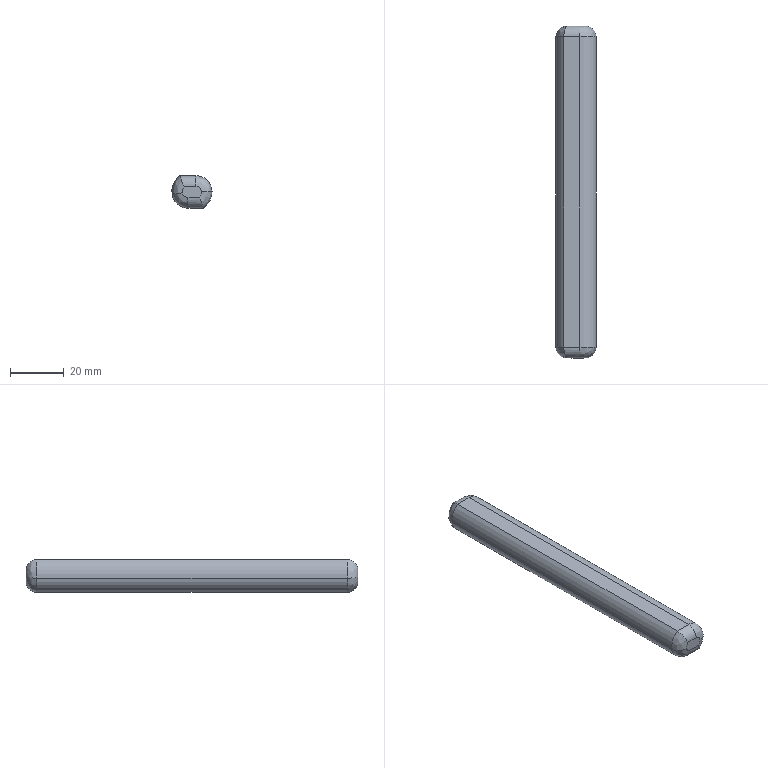Part | STEP file | solid 21 | 1 solid | 20 faces | box 15 x 124 x 12.156 mm | volume 19013 mm3 | cylinder 8 | spline 8 | plane 4 | commonest cylinder face diameters 8 x4 12 x2 15 x2